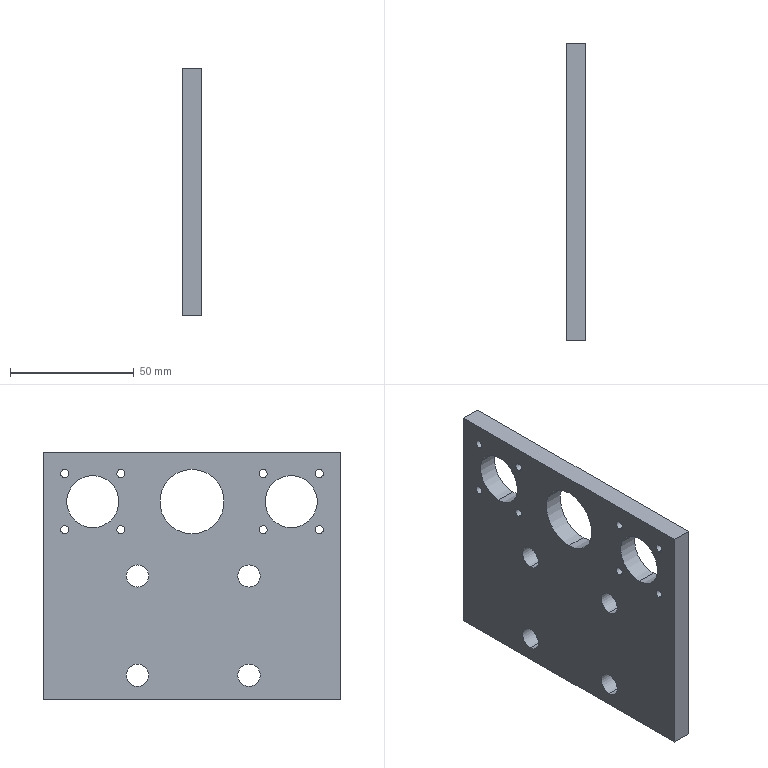Part | STEP file | X77B-01003 | 1 solid | 36 faces | box 8 x 120 x 100 mm | volume 83628 mm3 | cylinder 30 | plane 6 | commonest cylinder face diameters 3.3 x16 9 x8 21 x4 26 x2
STEP:
#1=CARTESIAN_POINT('',(289.016,-150.693,14.5));
#2=VERTEX_POINT('',#1);
#3=CARTESIAN_POINT('',(289.016,-150.693,5.5));
#4=VERTEX_POINT('',#3);
#5=CARTESIAN_POINT('',(289.016,-150.693,10.));
#6=DIRECTION('',(1.,0.,0.));
#7=DIRECTION('',(0.,0.,-1.));
#8=AXIS2_PLACEMENT_3D('',#5,#6,#7);
#9=CIRCLE('',#8,4.5);
#10=EDGE_CURVE('',#2,#4,#9,.T.);
#11=ORIENTED_EDGE('',*,*,#10,.F.);
#12=CARTESIAN_POINT('',(297.016,-150.693,14.5));
#13=VERTEX_POINT('',#12);
#14=CARTESIAN_POINT('',(297.016,-150.693,14.5));
#15=DIRECTION('',(1.,0.,0.));
#16=VECTOR('',#15,1000.);
#17=LINE('',#14,#16);
#18=EDGE_CURVE('',#2,#13,#17,.T.);
#19=ORIENTED_EDGE('',*,*,#18,.T.);
#20=CARTESIAN_POINT('',(297.016,-150.693,5.5));
#21=VERTEX_POINT('',#20);
#22=CARTESIAN_POINT('',(297.016,-150.693,10.));
#23=DIRECTION('',(1.,0.,0.));
#24=DIRECTION('',(0.,0.,-1.));
#25=AXIS2_PLACEMENT_3D('',#22,#23,#24);
#26=CIRCLE('',#25,4.5);
#27=EDGE_CURVE('',#13,#21,#26,.T.);
#28=ORIENTED_EDGE('',*,*,#27,.T.);
#29=CARTESIAN_POINT('',(297.016,-150.693,5.5));
#30=DIRECTION('',(1.,0.,0.));
#31=VECTOR('',#30,1000.);
#32=LINE('',#29,#31);
#33=EDGE_CURVE('',#4,#21,#32,.T.);
#34=ORIENTED_EDGE('',*,*,#33,.F.);
#35=EDGE_LOOP('',(#11,#19,#28,#34));
#36=FACE_OUTER_BOUND('',#35,.T.);
#37=CARTESIAN_POINT('',(297.016,-150.693,10.));
#38=DIRECTION('',(1.,0.,0.));
#39=DIRECTION('',(0.,0.,-1.));
#40=AXIS2_PLACEMENT_3D('',#37,#38,#39);
#41=CYLINDRICAL_SURFACE('',#40,4.5);
#42=ADVANCED_FACE('',(#36),#41,.F.);
#43=CARTESIAN_POINT('',(289.016,-150.693,54.5));
#44=VERTEX_POINT('',#43);
#45=CARTESIAN_POINT('',(289.016,-150.693,45.5));
#46=VERTEX_POINT('',#45);
#47=CARTESIAN_POINT('',(289.016,-150.693,50.));
#48=DIRECTION('',(1.,0.,0.));
#49=DIRECTION('',(0.,0.,-1.));
#50=AXIS2_PLACEMENT_3D('',#47,#48,#49);
#51=CIRCLE('',#50,4.5);
#52=EDGE_CURVE('',#44,#46,#51,.T.);
#53=ORIENTED_EDGE('',*,*,#52,.F.);
#54=CARTESIAN_POINT('',(297.016,-150.693,54.5));
#55=VERTEX_POINT('',#54);
#56=CARTESIAN_POINT('',(297.016,-150.693,54.5));
#57=DIRECTION('',(1.,0.,0.));
#58=VECTOR('',#57,1000.);
#59=LINE('',#56,#58);
#60=EDGE_CURVE('',#44,#55,#59,.T.);
#61=ORIENTED_EDGE('',*,*,#60,.T.);
#62=CARTESIAN_POINT('',(297.016,-150.693,45.5));
#63=VERTEX_POINT('',#62);
#64=CARTESIAN_POINT('',(297.016,-150.693,50.));
#65=DIRECTION('',(1.,0.,0.));
#66=DIRECTION('',(0.,0.,-1.));
#67=AXIS2_PLACEMENT_3D('',#64,#65,#66);
#68=CIRCLE('',#67,4.5);
#69=EDGE_CURVE('',#55,#63,#68,.T.);
#70=ORIENTED_EDGE('',*,*,#69,.T.);
#71=CARTESIAN_POINT('',(297.016,-150.693,45.5));
#72=DIRECTION('',(1.,0.,0.));
#73=VECTOR('',#72,1000.);
#74=LINE('',#71,#73);
#75=EDGE_CURVE('',#46,#63,#74,.T.);
#76=ORIENTED_EDGE('',*,*,#75,.F.);
#77=EDGE_LOOP('',(#53,#61,#70,#76));
#78=FACE_OUTER_BOUND('',#77,.T.);
#79=CARTESIAN_POINT('',(297.016,-150.693,50.));
#80=DIRECTION('',(1.,0.,0.));
#81=DIRECTION('',(0.,0.,-1.));
#82=AXIS2_PLACEMENT_3D('',#79,#80,#81);
#83=CYLINDRICAL_SURFACE('',#82,4.5);
#84=ADVANCED_FACE('',(#78),#83,.F.);
#85=CARTESIAN_POINT('',(289.016,-105.693,14.5));
#86=VERTEX_POINT('',#85);
#87=CARTESIAN_POINT('',(289.016,-105.693,5.5));
#88=VERTEX_POINT('',#87);
#89=CARTESIAN_POINT('',(289.016,-105.693,10.));
#90=DIRECTION('',(1.,0.,0.));
#91=DIRECTION('',(0.,0.,-1.));
#92=AXIS2_PLACEMENT_3D('',#89,#90,#91);
#93=CIRCLE('',#92,4.5);
#94=EDGE_CURVE('',#86,#88,#93,.T.);
#95=ORIENTED_EDGE('',*,*,#94,.F.);
#96=CARTESIAN_POINT('',(297.016,-105.693,14.5));
#97=VERTEX_POINT('',#96);
#98=CARTESIAN_POINT('',(297.016,-105.693,14.5));
#99=DIRECTION('',(1.,0.,0.));
#100=VECTOR('',#99,1000.);
#101=LINE('',#98,#100);
#102=EDGE_CURVE('',#86,#97,#101,.T.);
#103=ORIENTED_EDGE('',*,*,#102,.T.);
#104=CARTESIAN_POINT('',(297.016,-105.693,5.5));
#105=VERTEX_POINT('',#104);
#106=CARTESIAN_POINT('',(297.016,-105.693,10.));
#107=DIRECTION('',(1.,0.,0.));
#108=DIRECTION('',(0.,0.,-1.));
#109=AXIS2_PLACEMENT_3D('',#106,#107,#108);
#110=CIRCLE('',#109,4.5);
#111=EDGE_CURVE('',#97,#105,#110,.T.);
#112=ORIENTED_EDGE('',*,*,#111,.T.);
#113=CARTESIAN_POINT('',(297.016,-105.693,5.5));
#114=DIRECTION('',(1.,0.,0.));
#115=VECTOR('',#114,1000.);
#116=LINE('',#113,#115);
#117=EDGE_CURVE('',#88,#105,#116,.T.);
#118=ORIENTED_EDGE('',*,*,#117,.F.);
#119=EDGE_LOOP('',(#95,#103,#112,#118));
#120=FACE_OUTER_BOUND('',#119,.T.);
#121=CARTESIAN_POINT('',(297.016,-105.693,10.));
#122=DIRECTION('',(1.,0.,0.));
#123=DIRECTION('',(0.,0.,-1.));
#124=AXIS2_PLACEMENT_3D('',#121,#122,#123);
#125=CYLINDRICAL_SURFACE('',#124,4.5);
#126=ADVANCED_FACE('',(#120),#125,.F.);
#127=CARTESIAN_POINT('',(289.016,-105.693,54.5));
#128=VERTEX_POINT('',#127);
#129=CARTESIAN_POINT('',(289.016,-105.693,45.5));
#130=VERTEX_POINT('',#129);
#131=CARTESIAN_POINT('',(289.016,-105.693,50.));
#132=DIRECTION('',(1.,0.,0.));
#133=DIRECTION('',(0.,0.,-1.));
#134=AXIS2_PLACEMENT_3D('',#131,#132,#133);
#135=CIRCLE('',#134,4.5);
#136=EDGE_CURVE('',#128,#130,#135,.T.);
#137=ORIENTED_EDGE('',*,*,#136,.F.);
#138=CARTESIAN_POINT('',(297.016,-105.693,54.5));
#139=VERTEX_POINT('',#138);
#140=CARTESIAN_POINT('',(297.016,-105.693,54.5));
#141=DIRECTION('',(1.,0.,0.));
#142=VECTOR('',#141,1000.);
#143=LINE('',#140,#142);
#144=EDGE_CURVE('',#128,#139,#143,.T.);
#145=ORIENTED_EDGE('',*,*,#144,.T.);
#146=CARTESIAN_POINT('',(297.016,-105.693,45.5));
#147=VERTEX_POINT('',#146);
#148=CARTESIAN_POINT('',(297.016,-105.693,50.));
#149=DIRECTION('',(1.,0.,0.));
#150=DIRECTION('',(0.,0.,-1.));
#151=AXIS2_PLACEMENT_3D('',#148,#149,#150);
#152=CIRCLE('',#151,4.5);
#153=EDGE_CURVE('',#139,#147,#152,.T.);
#154=ORIENTED_EDGE('',*,*,#153,.T.);
#155=CARTESIAN_POINT('',(297.016,-105.693,45.5));
#156=DIRECTION('',(1.,0.,0.));
#157=VECTOR('',#156,1000.);
#158=LINE('',#155,#157);
#159=EDGE_CURVE('',#130,#147,#158,.T.);
#160=ORIENTED_EDGE('',*,*,#159,.F.);
#161=EDGE_LOOP('',(#137,#145,#154,#160));
#162=FACE_OUTER_BOUND('',#161,.T.);
#163=CARTESIAN_POINT('',(297.016,-105.693,50.));
#164=DIRECTION('',(1.,0.,0.));
#165=DIRECTION('',(0.,0.,-1.));
#166=AXIS2_PLACEMENT_3D('',#163,#164,#165);
#167=CYLINDRICAL_SURFACE('',#166,4.5);
#168=ADVANCED_FACE('',(#162),#167,.F.);
#169=CARTESIAN_POINT('',(289.016,-76.387,70.336));
#170=VERTEX_POINT('',#169);
#171=CARTESIAN_POINT('',(289.016,-76.387,67.036));
#172=VERTEX_POINT('',#171);
#173=CARTESIAN_POINT('',(289.016,-76.387,68.686));
#174=DIRECTION('',(1.,0.,0.));
#175=DIRECTION('',(0.,0.,-1.));
#176=AXIS2_PLACEMENT_3D('',#173,#174,#175);
#177=CIRCLE('',#176,1.65);
#178=EDGE_CURVE('',#170,#172,#177,.T.);
#179=ORIENTED_EDGE('',*,*,#178,.F.);
#180=CARTESIAN_POINT('',(297.016,-76.387,70.336));
#181=VERTEX_POINT('',#180);
#182=CARTESIAN_POINT('',(297.016,-76.387,70.336));
#183=DIRECTION('',(1.,0.,0.));
#184=VECTOR('',#183,1000.);
#185=LINE('',#182,#184);
#186=EDGE_CURVE('',#170,#181,#185,.T.);
#187=ORIENTED_EDGE('',*,*,#186,.T.);
#188=CARTESIAN_POINT('',(297.016,-76.387,67.036));
#189=VERTEX_POINT('',#188);
#190=CARTESIAN_POINT('',(297.016,-76.387,68.686));
#191=DIRECTION('',(1.,0.,0.));
#192=DIRECTION('',(0.,0.,-1.));
#193=AXIS2_PLACEMENT_3D('',#190,#191,#192);
#194=CIRCLE('',#193,1.65);
#195=EDGE_CURVE('',#181,#189,#194,.T.);
#196=ORIENTED_EDGE('',*,*,#195,.T.);
#197=CARTESIAN_POINT('',(297.016,-76.387,67.036));
#198=DIRECTION('',(1.,0.,0.));
#199=VECTOR('',#198,1000.);
#200=LINE('',#197,#199);
#201=EDGE_CURVE('',#172,#189,#200,.T.);
#202=ORIENTED_EDGE('',*,*,#201,.F.);
#203=EDGE_LOOP('',(#179,#187,#196,#202));
#204=FACE_OUTER_BOUND('',#203,.T.);
#205=CARTESIAN_POINT('',(297.016,-76.387,68.686));
#206=DIRECTION('',(1.,0.,0.));
#207=DIRECTION('',(0.,0.,-1.));
#208=AXIS2_PLACEMENT_3D('',#205,#206,#207);
#209=CYLINDRICAL_SURFACE('',#208,1.65);
#210=ADVANCED_FACE('',(#204),#209,.F.);
#211=CARTESIAN_POINT('',(289.016,-99.014,70.336));
#212=VERTEX_POINT('',#211);
#213=CARTESIAN_POINT('',(289.016,-99.014,67.036));
#214=VERTEX_POINT('',#213);
#215=CARTESIAN_POINT('',(289.016,-99.014,68.686));
#216=DIRECTION('',(1.,0.,0.));
#217=DIRECTION('',(0.,0.,-1.));
#218=AXIS2_PLACEMENT_3D('',#215,#216,#217);
#219=CIRCLE('',#218,1.65);
#220=EDGE_CURVE('',#212,#214,#219,.T.);
#221=ORIENTED_EDGE('',*,*,#220,.F.);
#222=CARTESIAN_POINT('',(297.016,-99.014,70.336));
#223=VERTEX_POINT('',#222);
#224=CARTESIAN_POINT('',(297.016,-99.014,70.336));
#225=DIRECTION('',(1.,0.,0.));
#226=VECTOR('',#225,1000.);
#227=LINE('',#224,#226);
#228=EDGE_CURVE('',#212,#223,#227,.T.);
#229=ORIENTED_EDGE('',*,*,#228,.T.);
#230=CARTESIAN_POINT('',(297.016,-99.014,67.036));
#231=VERTEX_POINT('',#230);
#232=CARTESIAN_POINT('',(297.016,-99.014,68.686));
#233=DIRECTION('',(1.,0.,0.));
#234=DIRECTION('',(0.,0.,-1.));
#235=AXIS2_PLACEMENT_3D('',#232,#233,#234);
#236=CIRCLE('',#235,1.65);
#237=EDGE_CURVE('',#223,#231,#236,.T.);
#238=ORIENTED_EDGE('',*,*,#237,.T.);
#239=CARTESIAN_POINT('',(297.016,-99.014,67.036));
#240=DIRECTION('',(1.,0.,0.));
#241=VECTOR('',#240,1000.);
#242=LINE('',#239,#241);
#243=EDGE_CURVE('',#214,#231,#242,.T.);
#244=ORIENTED_EDGE('',*,*,#243,.F.);
#245=EDGE_LOOP('',(#221,#229,#238,#244));
#246=FACE_OUTER_BOUND('',#245,.T.);
#247=CARTESIAN_POINT('',(297.016,-99.014,68.686));
#248=DIRECTION('',(1.,0.,0.));
#249=DIRECTION('',(0.,0.,-1.));
#250=AXIS2_PLACEMENT_3D('',#247,#248,#249);
#251=CYLINDRICAL_SURFACE('',#250,1.65);
#252=ADVANCED_FACE('',(#246),#251,.F.);
#253=CARTESIAN_POINT('',(289.016,-76.387,92.964));
#254=VERTEX_POINT('',#253);
#255=CARTESIAN_POINT('',(289.016,-76.387,89.664));
#256=VERTEX_POINT('',#255);
#257=CARTESIAN_POINT('',(289.016,-76.387,91.314));
#258=DIRECTION('',(1.,0.,0.));
#259=DIRECTION('',(0.,0.,-1.));
#260=AXIS2_PLACEMENT_3D('',#257,#258,#259);
#261=CIRCLE('',#260,1.65);
#262=EDGE_CURVE('',#254,#256,#261,.T.);
#263=ORIENTED_EDGE('',*,*,#262,.F.);
#264=CARTESIAN_POINT('',(297.016,-76.387,92.964));
#265=VERTEX_POINT('',#264);
#266=CARTESIAN_POINT('',(297.016,-76.387,92.964));
#267=DIRECTION('',(1.,0.,0.));
#268=VECTOR('',#267,1000.);
#269=LINE('',#266,#268);
#270=EDGE_CURVE('',#254,#265,#269,.T.);
#271=ORIENTED_EDGE('',*,*,#270,.T.);
#272=CARTESIAN_POINT('',(297.016,-76.387,89.664));
#273=VERTEX_POINT('',#272);
#274=CARTESIAN_POINT('',(297.016,-76.387,91.314));
#275=DIRECTION('',(1.,0.,0.));
#276=DIRECTION('',(0.,0.,-1.));
#277=AXIS2_PLACEMENT_3D('',#274,#275,#276);
#278=CIRCLE('',#277,1.65);
#279=EDGE_CURVE('',#265,#273,#278,.T.);
#280=ORIENTED_EDGE('',*,*,#279,.T.);
#281=CARTESIAN_POINT('',(297.016,-76.387,89.664));
#282=DIRECTION('',(1.,0.,0.));
#283=VECTOR('',#282,1000.);
#284=LINE('',#281,#283);
#285=EDGE_CURVE('',#256,#273,#284,.T.);
#286=ORIENTED_EDGE('',*,*,#285,.F.);
#287=EDGE_LOOP('',(#263,#271,#280,#286));
#288=FACE_OUTER_BOUND('',#287,.T.);
#289=CARTESIAN_POINT('',(297.016,-76.387,91.314));
#290=DIRECTION('',(1.,0.,0.));
#291=DIRECTION('',(0.,0.,-1.));
#292=AXIS2_PLACEMENT_3D('',#289,#290,#291);
#293=CYLINDRICAL_SURFACE('',#292,1.65);
#294=ADVANCED_FACE('',(#288),#293,.F.);
#295=CARTESIAN_POINT('',(289.016,-99.014,92.964));
#296=VERTEX_POINT('',#295);
#297=CARTESIAN_POINT('',(289.016,-99.014,89.664));
#298=VERTEX_POINT('',#297);
#299=CARTESIAN_POINT('',(289.016,-99.014,91.314));
#300=DIRECTION('',(1.,0.,0.));
#301=DIRECTION('',(0.,0.,-1.));
#302=AXIS2_PLACEMENT_3D('',#299,#300,#301);
#303=CIRCLE('',#302,1.65);
#304=EDGE_CURVE('',#296,#298,#303,.T.);
#305=ORIENTED_EDGE('',*,*,#304,.F.);
#306=CARTESIAN_POINT('',(297.016,-99.014,92.964));
#307=VERTEX_POINT('',#306);
#308=CARTESIAN_POINT('',(297.016,-99.014,92.964));
#309=DIRECTION('',(1.,0.,0.));
#310=VECTOR('',#309,1000.);
#311=LINE('',#308,#310);
#312=EDGE_CURVE('',#296,#307,#311,.T.);
#313=ORIENTED_EDGE('',*,*,#312,.T.);
#314=CARTESIAN_POINT('',(297.016,-99.014,89.664));
#315=VERTEX_POINT('',#314);
#316=CARTESIAN_POINT('',(297.016,-99.014,91.314));
#317=DIRECTION('',(1.,0.,0.));
#318=DIRECTION('',(0.,0.,-1.));
#319=AXIS2_PLACEMENT_3D('',#316,#317,#318);
#320=CIRCLE('',#319,1.65);
#321=EDGE_CURVE('',#307,#315,#320,.T.);
#322=ORIENTED_EDGE('',*,*,#321,.T.);
#323=CARTESIAN_POINT('',(297.016,-99.014,89.664));
#324=DIRECTION('',(1.,0.,0.));
#325=VECTOR('',#324,1000.);
#326=LINE('',#323,#325);
#327=EDGE_CURVE('',#298,#315,#326,.T.);
#328=ORIENTED_EDGE('',*,*,#327,.F.);
#329=EDGE_LOOP('',(#305,#313,#322,#328));
#330=FACE_OUTER_BOUND('',#329,.T.);
#331=CARTESIAN_POINT('',(297.016,-99.014,91.314));
#332=DIRECTION('',(1.,0.,0.));
#333=DIRECTION('',(0.,0.,-1.));
#334=AXIS2_PLACEMENT_3D('',#331,#332,#333);
#335=CYLINDRICAL_SURFACE('',#334,1.65);
#336=ADVANCED_FACE('',(#330),#335,.F.);
#337=CARTESIAN_POINT('',(289.016,-156.401,70.336));
#338=VERTEX_POINT('',#337);
#339=CARTESIAN_POINT('',(289.016,-156.401,67.036));
#340=VERTEX_POINT('',#339);
#341=CARTESIAN_POINT('',(289.016,-156.401,68.686));
#342=DIRECTION('',(1.,0.,0.));
#343=DIRECTION('',(0.,0.,-1.));
#344=AXIS2_PLACEMENT_3D('',#341,#342,#343);
#345=CIRCLE('',#344,1.65);
#346=EDGE_CURVE('',#338,#340,#345,.T.);
#347=ORIENTED_EDGE('',*,*,#346,.F.);
#348=CARTESIAN_POINT('',(297.016,-156.401,70.336));
#349=VERTEX_POINT('',#348);
#350=CARTESIAN_POINT('',(297.016,-156.401,70.336));
#351=DIRECTION('',(1.,0.,0.));
#352=VECTOR('',#351,1000.);
#353=LINE('',#350,#352);
#354=EDGE_CURVE('',#338,#349,#353,.T.);
#355=ORIENTED_EDGE('',*,*,#354,.T.);
#356=CARTESIAN_POINT('',(297.016,-156.401,67.036));
#357=VERTEX_POINT('',#356);
#358=CARTESIAN_POINT('',(297.016,-156.401,68.686));
#359=DIRECTION('',(1.,0.,0.));
#360=DIRECTION('',(0.,0.,-1.));
#361=AXIS2_PLACEMENT_3D('',#358,#359,#360);
#362=CIRCLE('',#361,1.65);
#363=EDGE_CURVE('',#349,#357,#362,.T.);
#364=ORIENTED_EDGE('',*,*,#363,.T.);
#365=CARTESIAN_POINT('',(297.016,-156.401,67.036));
#366=DIRECTION('',(1.,0.,0.));
#367=VECTOR('',#366,1000.);
#368=LINE('',#365,#367);
#369=EDGE_CURVE('',#340,#357,#368,.T.);
#370=ORIENTED_EDGE('',*,*,#369,.F.);
#371=EDGE_LOOP('',(#347,#355,#364,#370));
#372=FACE_OUTER_BOUND('',#371,.T.);
#373=CARTESIAN_POINT('',(297.016,-156.401,68.686));
#374=DIRECTION('',(1.,0.,0.));
#375=DIRECTION('',(0.,0.,-1.));
#376=AXIS2_PLACEMENT_3D('',#373,#374,#375);
#377=CYLINDRICAL_SURFACE('',#376,1.65);
#378=ADVANCED_FACE('',(#372),#377,.F.);
#379=CARTESIAN_POINT('',(289.016,-156.401,92.964));
#380=VERTEX_POINT('',#379);
#381=CARTESIAN_POINT('',(289.016,-156.401,89.664));
#382=VERTEX_POINT('',#381);
#383=CARTESIAN_POINT('',(289.016,-156.401,91.314));
#384=DIRECTION('',(1.,0.,0.));
#385=DIRECTION('',(0.,0.,-1.));
#386=AXIS2_PLACEMENT_3D('',#383,#384,#385);
#387=CIRCLE('',#386,1.65);
#388=EDGE_CURVE('',#380,#382,#387,.T.);
#389=ORIENTED_EDGE('',*,*,#388,.F.);
#390=CARTESIAN_POINT('',(297.016,-156.401,92.964));
#391=VERTEX_POINT('',#390);
#392=CARTESIAN_POINT('',(297.016,-156.401,92.964));
#393=DIRECTION('',(1.,0.,0.));
#394=VECTOR('',#393,1000.);
#395=LINE('',#392,#394);
#396=EDGE_CURVE('',#380,#391,#395,.T.);
#397=ORIENTED_EDGE('',*,*,#396,.T.);
#398=CARTESIAN_POINT('',(297.016,-156.401,89.664));
#399=VERTEX_POINT('',#398);
#400=CARTESIAN_POINT('',(297.016,-156.401,91.314));
#401=DIRECTION('',(1.,0.,0.));
#402=DIRECTION('',(0.,0.,-1.));
#403=AXIS2_PLACEMENT_3D('',#400,#401,#402);
#404=CIRCLE('',#403,1.65);
#405=EDGE_CURVE('',#391,#399,#404,.T.);
#406=ORIENTED_EDGE('',*,*,#405,.T.);
#407=CARTESIAN_POINT('',(297.016,-156.401,89.664));
#408=DIRECTION('',(1.,0.,0.));
#409=VECTOR('',#408,1000.);
#410=LINE('',#407,#409);
#411=EDGE_CURVE('',#382,#399,#410,.T.);
#412=ORIENTED_EDGE('',*,*,#411,.F.);
#413=EDGE_LOOP('',(#389,#397,#406,#412));
#414=FACE_OUTER_BOUND('',#413,.T.);
#415=CARTESIAN_POINT('',(297.016,-156.401,91.314));
#416=DIRECTION('',(1.,0.,0.));
#417=DIRECTION('',(0.,0.,-1.));
#418=AXIS2_PLACEMENT_3D('',#415,#416,#417);
#419=CYLINDRICAL_SURFACE('',#418,1.65);
#420=ADVANCED_FACE('',(#414),#419,.F.);
#421=CARTESIAN_POINT('',(289.016,-179.028,92.964));
#422=VERTEX_POINT('',#421);
#423=CARTESIAN_POINT('',(289.016,-179.028,89.664));
#424=VERTEX_POINT('',#423);
#425=CARTESIAN_POINT('',(289.016,-179.028,91.314));
#426=DIRECTION('',(1.,0.,0.));
#427=DIRECTION('',(0.,0.,-1.));
#428=AXIS2_PLACEMENT_3D('',#425,#426,#427);
#429=CIRCLE('',#428,1.65);
#430=EDGE_CURVE('',#422,#424,#429,.T.);
#431=ORIENTED_EDGE('',*,*,#430,.F.);
#432=CARTESIAN_POINT('',(297.016,-179.028,92.964));
#433=VERTEX_POINT('',#432);
#434=CARTESIAN_POINT('',(297.016,-179.028,92.964));
#435=DIRECTION('',(1.,0.,0.));
#436=VECTOR('',#435,1000.);
#437=LINE('',#434,#436);
#438=EDGE_CURVE('',#422,#433,#437,.T.);
#439=ORIENTED_EDGE('',*,*,#438,.T.);
#440=CARTESIAN_POINT('',(297.016,-179.028,89.664));
#441=VERTEX_POINT('',#440);
#442=CARTESIAN_POINT('',(297.016,-179.028,91.314));
#443=DIRECTION('',(1.,0.,0.));
#444=DIRECTION('',(0.,0.,-1.));
#445=AXIS2_PLACEMENT_3D('',#442,#443,#444);
#446=CIRCLE('',#445,1.65);
#447=EDGE_CURVE('',#433,#441,#446,.T.);
#448=ORIENTED_EDGE('',*,*,#447,.T.);
#449=CARTESIAN_POINT('',(297.016,-179.028,89.664));
#450=DIRECTION('',(1.,0.,0.));
#451=VECTOR('',#450,1000.);
#452=LINE('',#449,#451);
#453=EDGE_CURVE('',#424,#441,#452,.T.);
#454=ORIENTED_EDGE('',*,*,#453,.F.);
#455=EDGE_LOOP('',(#431,#439,#448,#454));
#456=FACE_OUTER_BOUND('',#455,.T.);
#457=CARTESIAN_POINT('',(297.016,-179.028,91.314));
#458=DIRECTION('',(1.,0.,0.));
#459=DIRECTION('',(0.,0.,-1.));
#460=AXIS2_PLACEMENT_3D('',#457,#458,#459);
#461=CYLINDRICAL_SURFACE('',#460,1.65);
#462=ADVANCED_FACE('',(#456),#461,.F.);
#463=CARTESIAN_POINT('',(289.016,-179.028,70.336));
#464=VERTEX_POINT('',#463);
#465=CARTESIAN_POINT('',(289.016,-179.028,67.036));
#466=VERTEX_POINT('',#465);
#467=CARTESIAN_POINT('',(289.016,-179.028,68.686));
#468=DIRECTION('',(1.,0.,0.));
#469=DIRECTION('',(0.,0.,-1.));
#470=AXIS2_PLACEMENT_3D('',#467,#468,#469);
#471=CIRCLE('',#470,1.65);
#472=EDGE_CURVE('',#464,#466,#471,.T.);
#473=ORIENTED_EDGE('',*,*,#472,.F.);
#474=CARTESIAN_POINT('',(297.016,-179.028,70.336));
#475=VERTEX_POINT('',#474);
#476=CARTESIAN_POINT('',(297.016,-179.028,70.336));
#477=DIRECTION('',(1.,0.,0.));
#478=VECTOR('',#477,1000.);
#479=LINE('',#476,#478);
#480=EDGE_CURVE('',#464,#475,#479,.T.);
#481=ORIENTED_EDGE('',*,*,#480,.T.);
#482=CARTESIAN_POINT('',(297.016,-179.028,67.036));
#483=VERTEX_POINT('',#482);
#484=CARTESIAN_POINT('',(297.016,-179.028,68.686));
#485=DIRECTION('',(1.,0.,0.));
#486=DIRECTION('',(0.,0.,-1.));
#487=AXIS2_PLACEMENT_3D('',#484,#485,#486);
#488=CIRCLE('',#487,1.65);
#489=EDGE_CURVE('',#475,#483,#488,.T.);
#490=ORIENTED_EDGE('',*,*,#489,.T.);
#491=CARTESIAN_POINT('',(297.016,-179.028,67.036));
#492=DIRECTION('',(1.,0.,0.));
#493=VECTOR('',#492,1000.);
#494=LINE('',#491,#493);
#495=EDGE_CURVE('',#466,#483,#494,.T.);
#496=ORIENTED_EDGE('',*,*,#495,.F.);
#497=EDGE_LOOP('',(#473,#481,#490,#496));
#498=FACE_OUTER_BOUND('',#497,.T.);
#499=CARTESIAN_POINT('',(297.016,-179.028,68.686));
#500=DIRECTION('',(1.,0.,0.));
#501=DIRECTION('',(0.,0.,-1.));
#502=AXIS2_PLACEMENT_3D('',#499,#500,#501);
#503=CYLINDRICAL_SURFACE('',#502,1.65);
#504=ADVANCED_FACE('',(#498),#503,.F.);
#505=CARTESIAN_POINT('',(289.016,-167.7,90.5));
#506=VERTEX_POINT('',#505);
#507=CARTESIAN_POINT('',(289.016,-167.7,69.5));
#508=VERTEX_POINT('',#507);
#509=CARTESIAN_POINT('',(289.016,-167.7,80.));
#510=DIRECTION('',(1.,0.,0.));
#511=DIRECTION('',(0.,0.,-1.));
#512=AXIS2_PLACEMENT_3D('',#509,#510,#511);
#513=CIRCLE('',#512,10.5);
#514=EDGE_CURVE('',#506,#508,#513,.T.);
#515=ORIENTED_EDGE('',*,*,#514,.F.);
#516=CARTESIAN_POINT('',(297.016,-167.7,90.5));
#517=VERTEX_POINT('',#516);
#518=CARTESIAN_POINT('',(289.016,-167.7,90.5));
#519=DIRECTION('',(1.,0.,0.));
#520=VECTOR('',#519,1000.);
#521=LINE('',#518,#520);
#522=EDGE_CURVE('',#506,#517,#521,.T.);
#523=ORIENTED_EDGE('',*,*,#522,.T.);
#524=CARTESIAN_POINT('',(297.016,-167.7,69.5));
#525=VERTEX_POINT('',#524);
#526=CARTESIAN_POINT('',(297.016,-167.7,80.));
#527=DIRECTION('',(1.,0.,0.));
#528=DIRECTION('',(0.,0.,-1.));
#529=AXIS2_PLACEMENT_3D('',#526,#527,#528);
#530=CIRCLE('',#529,10.5);
#531=EDGE_CURVE('',#517,#525,#530,.T.);
#532=ORIENTED_EDGE('',*,*,#531,.T.);
#533=CARTESIAN_POINT('',(289.016,-167.7,69.5));
#534=DIRECTION('',(1.,0.,0.));
#535=VECTOR('',#534,1000.);
#536=LINE('',#533,#535);
#537=EDGE_CURVE('',#508,#525,#536,.T.);
#538=ORIENTED_EDGE('',*,*,#537,.F.);
#539=EDGE_LOOP('',(#515,#523,#532,#538));
#540=FACE_OUTER_BOUND('',#539,.T.);
#541=CARTESIAN_POINT('',(289.016,-167.7,80.));
#542=DIRECTION('',(1.,0.,0.));
#543=DIRECTION('',(0.,0.,-1.));
#544=AXIS2_PLACEMENT_3D('',#541,#542,#543);
#545=CYLINDRICAL_SURFACE('',#544,10.5);
#546=ADVANCED_FACE('',(#540),#545,.F.);
#547=CARTESIAN_POINT('',(289.016,-87.7,90.5));
#548=VERTEX_POINT('',#547);
#549=CARTESIAN_POINT('',(289.016,-87.7,69.5));
#550=VERTEX_POINT('',#549);
#551=CARTESIAN_POINT('',(289.016,-87.7,80.));
#552=DIRECTION('',(1.,0.,0.));
#553=DIRECTION('',(0.,0.,-1.));
#554=AXIS2_PLACEMENT_3D('',#551,#552,#553);
#555=CIRCLE('',#554,10.5);
#556=EDGE_CURVE('',#548,#550,#555,.T.);
#557=ORIENTED_EDGE('',*,*,#556,.F.);
#558=CARTESIAN_POINT('',(297.016,-87.7,90.5));
#559=VERTEX_POINT('',#558);
#560=CARTESIAN_POINT('',(289.016,-87.7,90.5));
#561=DIRECTION('',(1.,0.,0.));
#562=VECTOR('',#561,1000.);
#563=LINE('',#560,#562);
#564=EDGE_CURVE('',#548,#559,#563,.T.);
#565=ORIENTED_EDGE('',*,*,#564,.T.);
#566=CARTESIAN_POINT('',(297.016,-87.7,69.5));
#567=VERTEX_POINT('',#566);
#568=CARTESIAN_POINT('',(297.016,-87.7,80.));
#569=DIRECTION('',(1.,0.,0.));
#570=DIRECTION('',(0.,0.,-1.));
#571=AXIS2_PLACEMENT_3D('',#568,#569,#570);
#572=CIRCLE('',#571,10.5);
#573=EDGE_CURVE('',#559,#567,#572,.T.);
#574=ORIENTED_EDGE('',*,*,#573,.T.);
#575=CARTESIAN_POINT('',(289.016,-87.7,69.5));
#576=DIRECTION('',(1.,0.,0.));
#577=VECTOR('',#576,1000.);
#578=LINE('',#575,#577);
#579=EDGE_CURVE('',#550,#567,#578,.T.);
#580=ORIENTED_EDGE('',*,*,#579,.F.);
#581=EDGE_LOOP('',(#557,#565,#574,#580));
#582=FACE_OUTER_BOUND('',#581,.T.);
#583=CARTESIAN_POINT('',(289.016,-87.7,80.));
#584=DIRECTION('',(1.,0.,0.));
#585=DIRECTION('',(0.,0.,-1.));
#586=AXIS2_PLACEMENT_3D('',#583,#584,#585);
#587=CYLINDRICAL_SURFACE('',#586,10.5);
#588=ADVANCED_FACE('',(#582),#587,.F.);
#589=CARTESIAN_POINT('',(289.016,-127.7,93.));
#590=VERTEX_POINT('',#589);
#591=CARTESIAN_POINT('',(289.016,-127.7,67.));
#592=VERTEX_POINT('',#591);
#593=CARTESIAN_POINT('',(289.016,-127.7,80.));
#594=DIRECTION('',(1.,0.,0.));
#595=DIRECTION('',(0.,0.,-1.));
#596=AXIS2_PLACEMENT_3D('',#593,#594,#595);
#597=CIRCLE('',#596,13.);
#598=EDGE_CURVE('',#590,#592,#597,.T.);
#599=ORIENTED_EDGE('',*,*,#598,.F.);
#600=CARTESIAN_POINT('',(297.016,-127.7,93.));
#601=VERTEX_POINT('',#600);
#602=CARTESIAN_POINT('',(289.016,-127.7,93.));
#603=DIRECTION('',(1.,0.,0.));
#604=VECTOR('',#603,1000.);
#605=LINE('',#602,#604);
#606=EDGE_CURVE('',#590,#601,#605,.T.);
#607=ORIENTED_EDGE('',*,*,#606,.T.);
#608=CARTESIAN_POINT('',(297.016,-127.7,67.));
#609=VERTEX_POINT('',#608);
#610=CARTESIAN_POINT('',(297.016,-127.7,80.));
#611=DIRECTION('',(1.,0.,0.));
#612=DIRECTION('',(0.,0.,-1.));
#613=AXIS2_PLACEMENT_3D('',#610,#611,#612);
#614=CIRCLE('',#613,13.);
#615=EDGE_CURVE('',#601,#609,#614,.T.);
#616=ORIENTED_EDGE('',*,*,#615,.T.);
#617=CARTESIAN_POINT('',(289.016,-127.7,67.));
#618=DIRECTION('',(1.,0.,0.));
#619=VECTOR('',#618,1000.);
#620=LINE('',#617,#619);
#621=EDGE_CURVE('',#592,#609,#620,.T.);
#622=ORIENTED_EDGE('',*,*,#621,.F.);
#623=EDGE_LOOP('',(#599,#607,#616,#622));
#624=FACE_OUTER_BOUND('',#623,.T.);
#625=CARTESIAN_POINT('',(289.016,-127.7,80.));
#626=DIRECTION('',(1.,0.,0.));
#627=DIRECTION('',(0.,0.,-1.));
#628=AXIS2_PLACEMENT_3D('',#625,#626,#627);
#629=CYLINDRICAL_SURFACE('',#628,13.);
#630=ADVANCED_FACE('',(#624),#629,.F.);
#631=CARTESIAN_POINT('',(297.016,-150.693,10.));
#632=DIRECTION('',(1.,0.,0.));
#633=DIRECTION('',(0.,0.,-1.));
#634=AXIS2_PLACEMENT_3D('',#631,#632,#633);
#635=CIRCLE('',#634,4.5);
#636=EDGE_CURVE('',#21,#13,#635,.T.);
#637=ORIENTED_EDGE('',*,*,#636,.F.);
#638=ORIENTED_EDGE('',*,*,#27,.F.);
#639=EDGE_LOOP('',(#637,#638));
#640=FACE_BOUND('',#639,.T.);
#641=CARTESIAN_POINT('',(297.016,-150.693,50.));
#642=DIRECTION('',(1.,0.,0.));
#643=DIRECTION('',(0.,0.,-1.));
#644=AXIS2_PLACEMENT_3D('',#641,#642,#643);
#645=CIRCLE('',#644,4.5);
#646=EDGE_CURVE('',#63,#55,#645,.T.);
#647=ORIENTED_EDGE('',*,*,#646,.F.);
#648=ORIENTED_EDGE('',*,*,#69,.F.);
#649=EDGE_LOOP('',(#647,#648));
#650=FACE_BOUND('',#649,.T.);
#651=CARTESIAN_POINT('',(297.016,-105.693,10.));
#652=DIRECTION('',(1.,0.,0.));
#653=DIRECTION('',(0.,0.,-1.));
#654=AXIS2_PLACEMENT_3D('',#651,#652,#653);
#655=CIRCLE('',#654,4.5);
#656=EDGE_CURVE('',#105,#97,#655,.T.);
#657=ORIENTED_EDGE('',*,*,#656,.F.);
#658=ORIENTED_EDGE('',*,*,#111,.F.);
#659=EDGE_LOOP('',(#657,#658));
#660=FACE_BOUND('',#659,.T.);
#661=CARTESIAN_POINT('',(297.016,-105.693,50.));
#662=DIRECTION('',(1.,0.,0.));
#663=DIRECTION('',(0.,0.,-1.));
#664=AXIS2_PLACEMENT_3D('',#661,#662,#663);
#665=CIRCLE('',#664,4.5);
#666=EDGE_CURVE('',#147,#139,#665,.T.);
#667=ORIENTED_EDGE('',*,*,#666,.F.);
#668=ORIENTED_EDGE('',*,*,#153,.F.);
#669=EDGE_LOOP('',(#667,#668));
#670=FACE_BOUND('',#669,.T.);
#671=CARTESIAN_POINT('',(297.016,-76.387,68.686));
#672=DIRECTION('',(1.,0.,0.));
#673=DIRECTION('',(0.,0.,-1.));
#674=AXIS2_PLACEMENT_3D('',#671,#672,#673);
#675=CIRCLE('',#674,1.65);
#676=EDGE_CURVE('',#189,#181,#675,.T.);
#677=ORIENTED_EDGE('',*,*,#676,.F.);
#678=ORIENTED_EDGE('',*,*,#195,.F.);
#679=EDGE_LOOP('',(#677,#678));
#680=FACE_BOUND('',#679,.T.);
#681=CARTESIAN_POINT('',(297.016,-99.014,68.686));
#682=DIRECTION('',(1.,0.,0.));
#683=DIRECTION('',(0.,0.,-1.));
#684=AXIS2_PLACEMENT_3D('',#681,#682,#683);
#685=CIRCLE('',#684,1.65);
#686=EDGE_CURVE('',#231,#223,#685,.T.);
#687=ORIENTED_EDGE('',*,*,#686,.F.);
#688=ORIENTED_EDGE('',*,*,#237,.F.);
#689=EDGE_LOOP('',(#687,#688));
#690=FACE_BOUND('',#689,.T.);
#691=CARTESIAN_POINT('',(297.016,-76.387,91.314));
#692=DIRECTION('',(1.,0.,0.));
#693=DIRECTION('',(0.,0.,-1.));
#694=AXIS2_PLACEMENT_3D('',#691,#692,#693);
#695=CIRCLE('',#694,1.65);
#696=EDGE_CURVE('',#273,#265,#695,.T.);
#697=ORIENTED_EDGE('',*,*,#696,.F.);
#698=ORIENTED_EDGE('',*,*,#279,.F.);
#699=EDGE_LOOP('',(#697,#698));
#700=FACE_BOUND('',#699,.T.);
#701=CARTESIAN_POINT('',(297.016,-99.014,91.314));
#702=DIRECTION('',(1.,0.,0.));
#703=DIRECTION('',(0.,0.,-1.));
#704=AXIS2_PLACEMENT_3D('',#701,#702,#703);
#705=CIRCLE('',#704,1.65);
#706=EDGE_CURVE('',#315,#307,#705,.T.);
#707=ORIENTED_EDGE('',*,*,#706,.F.);
#708=ORIENTED_EDGE('',*,*,#321,.F.);
#709=EDGE_LOOP('',(#707,#708));
#710=FACE_BOUND('',#709,.T.);
#711=CARTESIAN_POINT('',(297.016,-156.401,68.686));
#712=DIRECTION('',(1.,0.,0.));
#713=DIRECTION('',(0.,0.,-1.));
#714=AXIS2_PLACEMENT_3D('',#711,#712,#713);
#715=CIRCLE('',#714,1.65);
#716=EDGE_CURVE('',#357,#349,#715,.T.);
#717=ORIENTED_EDGE('',*,*,#716,.F.);
#718=ORIENTED_EDGE('',*,*,#363,.F.);
#719=EDGE_LOOP('',(#717,#718));
#720=FACE_BOUND('',#719,.T.);
#721=CARTESIAN_POINT('',(297.016,-156.401,91.314));
#722=DIRECTION('',(1.,0.,0.));
#723=DIRECTION('',(0.,0.,-1.));
#724=AXIS2_PLACEMENT_3D('',#721,#722,#723);
#725=CIRCLE('',#724,1.65);
#726=EDGE_CURVE('',#399,#391,#725,.T.);
#727=ORIENTED_EDGE('',*,*,#726,.F.);
#728=ORIENTED_EDGE('',*,*,#405,.F.);
#729=EDGE_LOOP('',(#727,#728));
#730=FACE_BOUND('',#729,.T.);
#731=CARTESIAN_POINT('',(297.016,-179.028,91.314));
#732=DIRECTION('',(1.,0.,0.));
#733=DIRECTION('',(0.,0.,-1.));
#734=AXIS2_PLACEMENT_3D('',#731,#732,#733);
#735=CIRCLE('',#734,1.65);
#736=EDGE_CURVE('',#441,#433,#735,.T.);
#737=ORIENTED_EDGE('',*,*,#736,.F.);
#738=ORIENTED_EDGE('',*,*,#447,.F.);
#739=EDGE_LOOP('',(#737,#738));
#740=FACE_BOUND('',#739,.T.);
#741=CARTESIAN_POINT('',(297.016,-179.028,68.686));
#742=DIRECTION('',(1.,0.,0.));
#743=DIRECTION('',(0.,0.,-1.));
#744=AXIS2_PLACEMENT_3D('',#741,#742,#743);
#745=CIRCLE('',#744,1.65);
#746=EDGE_CURVE('',#483,#475,#745,.T.);
#747=ORIENTED_EDGE('',*,*,#746,.F.);
#748=ORIENTED_EDGE('',*,*,#489,.F.);
#749=EDGE_LOOP('',(#747,#748));
#750=FACE_BOUND('',#749,.T.);
#751=CARTESIAN_POINT('',(297.016,-167.7,80.));
#752=DIRECTION('',(1.,0.,0.));
#753=DIRECTION('',(0.,0.,-1.));
#754=AXIS2_PLACEMENT_3D('',#751,#752,#753);
#755=CIRCLE('',#754,10.5);
#756=EDGE_CURVE('',#525,#517,#755,.T.);
#757=ORIENTED_EDGE('',*,*,#756,.F.);
#758=ORIENTED_EDGE('',*,*,#531,.F.);
#759=EDGE_LOOP('',(#757,#758));
#760=FACE_BOUND('',#759,.T.);
#761=CARTESIAN_POINT('',(297.016,-87.7,80.));
#762=DIRECTION('',(1.,0.,0.));
#763=DIRECTION('',(0.,0.,-1.));
#764=AXIS2_PLACEMENT_3D('',#761,#762,#763);
#765=CIRCLE('',#764,10.5);
#766=EDGE_CURVE('',#567,#559,#765,.T.);
#767=ORIENTED_EDGE('',*,*,#766,.F.);
#768=ORIENTED_EDGE('',*,*,#573,.F.);
#769=EDGE_LOOP('',(#767,#768));
#770=FACE_BOUND('',#769,.T.);
#771=CARTESIAN_POINT('',(297.016,-127.7,80.));
#772=DIRECTION('',(1.,0.,0.));
#773=DIRECTION('',(0.,0.,-1.));
#774=AXIS2_PLACEMENT_3D('',#771,#772,#773);
#775=CIRCLE('',#774,13.);
#776=EDGE_CURVE('',#609,#601,#775,.T.);
#777=ORIENTED_EDGE('',*,*,#776,.F.);
#778=ORIENTED_EDGE('',*,*,#615,.F.);
#779=EDGE_LOOP('',(#777,#778));
#780=FACE_BOUND('',#779,.T.);
#781=CARTESIAN_POINT('',(297.016,-187.7,0.));
#782=VERTEX_POINT('',#781);
#783=CARTESIAN_POINT('',(297.016,-67.7,0.));
#784=VERTEX_POINT('',#783);
#785=CARTESIAN_POINT('',(297.016,-67.7,0.));
#786=DIRECTION('',(0.,1.,0.));
#787=VECTOR('',#786,1000.);
#788=LINE('',#785,#787);
#789=EDGE_CURVE('',#782,#784,#788,.T.);
#790=ORIENTED_EDGE('',*,*,#789,.T.);
#791=CARTESIAN_POINT('',(297.016,-67.7,100.));
#792=VERTEX_POINT('',#791);
#793=CARTESIAN_POINT('',(297.016,-67.7,100.));
#794=DIRECTION('',(0.,0.,-1.));
#795=VECTOR('',#794,1000.);
#796=LINE('',#793,#795);
#797=EDGE_CURVE('',#792,#784,#796,.T.);
#798=ORIENTED_EDGE('',*,*,#797,.F.);
#799=CARTESIAN_POINT('',(297.016,-187.7,100.));
#800=VERTEX_POINT('',#799);
#801=CARTESIAN_POINT('',(297.016,-67.7,100.));
#802=DIRECTION('',(0.,1.,0.));
#803=VECTOR('',#802,1000.);
#804=LINE('',#801,#803);
#805=EDGE_CURVE('',#800,#792,#804,.T.);
#806=ORIENTED_EDGE('',*,*,#805,.F.);
#807=CARTESIAN_POINT('',(297.016,-187.7,100.));
#808=DIRECTION('',(0.,0.,-1.));
#809=VECTOR('',#808,1000.);
#810=LINE('',#807,#809);
#811=EDGE_CURVE('',#800,#782,#810,.T.);
#812=ORIENTED_EDGE('',*,*,#811,.T.);
#813=EDGE_LOOP('',(#790,#798,#806,#812));
#814=FACE_OUTER_BOUND('',#813,.T.);
#815=CARTESIAN_POINT('',(297.016,-67.7,100.));
#816=DIRECTION('',(-1.,0.,0.));
#817=DIRECTION('',(0.,0.,1.));
#818=AXIS2_PLACEMENT_3D('',#815,#816,#817);
#819=PLANE('',#818);
#820=ADVANCED_FACE('',(#640,#650,#660,#670,#680,#690,#700,#710,#720,#730,#740,#750,#760,#770,#780,#814),#819,.F.);
#821=CARTESIAN_POINT('',(289.016,-67.7,0.));
#822=VERTEX_POINT('',#821);
#823=CARTESIAN_POINT('',(297.016,-67.7,0.));
#824=DIRECTION('',(-1.,0.,0.));
#825=VECTOR('',#824,1000.);
#826=LINE('',#823,#825);
#827=EDGE_CURVE('',#784,#822,#826,.T.);
#828=ORIENTED_EDGE('',*,*,#827,.T.);
#829=CARTESIAN_POINT('',(289.016,-67.7,100.));
#830=VERTEX_POINT('',#829);
#831=CARTESIAN_POINT('',(289.016,-67.7,100.));
#832=DIRECTION('',(0.,0.,-1.));
#833=VECTOR('',#832,1000.);
#834=LINE('',#831,#833);
#835=EDGE_CURVE('',#830,#822,#834,.T.);
#836=ORIENTED_EDGE('',*,*,#835,.F.);
#837=CARTESIAN_POINT('',(297.016,-67.7,100.));
#838=DIRECTION('',(-1.,0.,0.));
#839=VECTOR('',#838,1000.);
#840=LINE('',#837,#839);
#841=EDGE_CURVE('',#792,#830,#840,.T.);
#842=ORIENTED_EDGE('',*,*,#841,.F.);
#843=ORIENTED_EDGE('',*,*,#797,.T.);
#844=EDGE_LOOP('',(#828,#836,#842,#843));
#845=FACE_OUTER_BOUND('',#844,.T.);
#846=CARTESIAN_POINT('',(297.016,-67.7,100.));
#847=DIRECTION('',(0.,-1.,0.));
#848=DIRECTION('',(0.,0.,-1.));
#849=AXIS2_PLACEMENT_3D('',#846,#847,#848);
#850=PLANE('',#849);
#851=ADVANCED_FACE('',(#845),#850,.F.);
#852=CARTESIAN_POINT('',(289.016,-150.693,10.));
#853=DIRECTION('',(1.,0.,0.));
#854=DIRECTION('',(0.,0.,-1.));
#855=AXIS2_PLACEMENT_3D('',#852,#853,#854);
#856=CIRCLE('',#855,4.5);
#857=EDGE_CURVE('',#4,#2,#856,.T.);
#858=ORIENTED_EDGE('',*,*,#857,.T.);
#859=ORIENTED_EDGE('',*,*,#10,.T.);
#860=EDGE_LOOP('',(#858,#859));
#861=FACE_BOUND('',#860,.T.);
#862=CARTESIAN_POINT('',(289.016,-150.693,50.));
#863=DIRECTION('',(1.,0.,0.));
#864=DIRECTION('',(0.,0.,-1.));
#865=AXIS2_PLACEMENT_3D('',#862,#863,#864);
#866=CIRCLE('',#865,4.5);
#867=EDGE_CURVE('',#46,#44,#866,.T.);
#868=ORIENTED_EDGE('',*,*,#867,.T.);
#869=ORIENTED_EDGE('',*,*,#52,.T.);
#870=EDGE_LOOP('',(#868,#869));
#871=FACE_BOUND('',#870,.T.);
#872=CARTESIAN_POINT('',(289.016,-105.693,10.));
#873=DIRECTION('',(1.,0.,0.));
#874=DIRECTION('',(0.,0.,-1.));
#875=AXIS2_PLACEMENT_3D('',#872,#873,#874);
#876=CIRCLE('',#875,4.5);
#877=EDGE_CURVE('',#88,#86,#876,.T.);
#878=ORIENTED_EDGE('',*,*,#877,.T.);
#879=ORIENTED_EDGE('',*,*,#94,.T.);
#880=EDGE_LOOP('',(#878,#879));
#881=FACE_BOUND('',#880,.T.);
#882=CARTESIAN_POINT('',(289.016,-105.693,50.));
#883=DIRECTION('',(1.,0.,0.));
#884=DIRECTION('',(0.,0.,-1.));
#885=AXIS2_PLACEMENT_3D('',#882,#883,#884);
#886=CIRCLE('',#885,4.5);
#887=EDGE_CURVE('',#130,#128,#886,.T.);
#888=ORIENTED_EDGE('',*,*,#887,.T.);
#889=ORIENTED_EDGE('',*,*,#136,.T.);
#890=EDGE_LOOP('',(#888,#889));
#891=FACE_BOUND('',#890,.T.);
#892=CARTESIAN_POINT('',(289.016,-76.387,68.686));
#893=DIRECTION('',(1.,0.,0.));
#894=DIRECTION('',(0.,0.,-1.));
#895=AXIS2_PLACEMENT_3D('',#892,#893,#894);
#896=CIRCLE('',#895,1.65);
#897=EDGE_CURVE('',#172,#170,#896,.T.);
#898=ORIENTED_EDGE('',*,*,#897,.T.);
#899=ORIENTED_EDGE('',*,*,#178,.T.);
#900=EDGE_LOOP('',(#898,#899));
#901=FACE_BOUND('',#900,.T.);
#902=CARTESIAN_POINT('',(289.016,-99.014,68.686));
#903=DIRECTION('',(1.,0.,0.));
#904=DIRECTION('',(0.,0.,-1.));
#905=AXIS2_PLACEMENT_3D('',#902,#903,#904);
#906=CIRCLE('',#905,1.65);
#907=EDGE_CURVE('',#214,#212,#906,.T.);
#908=ORIENTED_EDGE('',*,*,#907,.T.);
#909=ORIENTED_EDGE('',*,*,#220,.T.);
#910=EDGE_LOOP('',(#908,#909));
#911=FACE_BOUND('',#910,.T.);
#912=CARTESIAN_POINT('',(289.016,-76.387,91.314));
#913=DIRECTION('',(1.,0.,0.));
#914=DIRECTION('',(0.,0.,-1.));
#915=AXIS2_PLACEMENT_3D('',#912,#913,#914);
#916=CIRCLE('',#915,1.65);
#917=EDGE_CURVE('',#256,#254,#916,.T.);
#918=ORIENTED_EDGE('',*,*,#917,.T.);
#919=ORIENTED_EDGE('',*,*,#262,.T.);
#920=EDGE_LOOP('',(#918,#919));
#921=FACE_BOUND('',#920,.T.);
#922=CARTESIAN_POINT('',(289.016,-99.014,91.314));
#923=DIRECTION('',(1.,0.,0.));
#924=DIRECTION('',(0.,0.,-1.));
#925=AXIS2_PLACEMENT_3D('',#922,#923,#924);
#926=CIRCLE('',#925,1.65);
#927=EDGE_CURVE('',#298,#296,#926,.T.);
#928=ORIENTED_EDGE('',*,*,#927,.T.);
#929=ORIENTED_EDGE('',*,*,#304,.T.);
#930=EDGE_LOOP('',(#928,#929));
#931=FACE_BOUND('',#930,.T.);
#932=CARTESIAN_POINT('',(289.016,-156.401,68.686));
#933=DIRECTION('',(1.,0.,0.));
#934=DIRECTION('',(0.,0.,-1.));
#935=AXIS2_PLACEMENT_3D('',#932,#933,#934);
#936=CIRCLE('',#935,1.65);
#937=EDGE_CURVE('',#340,#338,#936,.T.);
#938=ORIENTED_EDGE('',*,*,#937,.T.);
#939=ORIENTED_EDGE('',*,*,#346,.T.);
#940=EDGE_LOOP('',(#938,#939));
#941=FACE_BOUND('',#940,.T.);
#942=CARTESIAN_POINT('',(289.016,-156.401,91.314));
#943=DIRECTION('',(1.,0.,0.));
#944=DIRECTION('',(0.,0.,-1.));
#945=AXIS2_PLACEMENT_3D('',#942,#943,#944);
#946=CIRCLE('',#945,1.65);
#947=EDGE_CURVE('',#382,#380,#946,.T.);
#948=ORIENTED_EDGE('',*,*,#947,.T.);
#949=ORIENTED_EDGE('',*,*,#388,.T.);
#950=EDGE_LOOP('',(#948,#949));
#951=FACE_BOUND('',#950,.T.);
#952=CARTESIAN_POINT('',(289.016,-179.028,91.314));
#953=DIRECTION('',(1.,0.,0.));
#954=DIRECTION('',(0.,0.,-1.));
#955=AXIS2_PLACEMENT_3D('',#952,#953,#954);
#956=CIRCLE('',#955,1.65);
#957=EDGE_CURVE('',#424,#422,#956,.T.);
#958=ORIENTED_EDGE('',*,*,#957,.T.);
#959=ORIENTED_EDGE('',*,*,#430,.T.);
#960=EDGE_LOOP('',(#958,#959));
#961=FACE_BOUND('',#960,.T.);
#962=CARTESIAN_POINT('',(289.016,-179.028,68.686));
#963=DIRECTION('',(1.,0.,0.));
#964=DIRECTION('',(0.,0.,-1.));
#965=AXIS2_PLACEMENT_3D('',#962,#963,#964);
#966=CIRCLE('',#965,1.65);
#967=EDGE_CURVE('',#466,#464,#966,.T.);
#968=ORIENTED_EDGE('',*,*,#967,.T.);
#969=ORIENTED_EDGE('',*,*,#472,.T.);
#970=EDGE_LOOP('',(#968,#969));
#971=FACE_BOUND('',#970,.T.);
#972=CARTESIAN_POINT('',(289.016,-167.7,80.));
#973=DIRECTION('',(1.,0.,0.));
#974=DIRECTION('',(0.,0.,-1.));
#975=AXIS2_PLACEMENT_3D('',#972,#973,#974);
#976=CIRCLE('',#975,10.5);
#977=EDGE_CURVE('',#508,#506,#976,.T.);
#978=ORIENTED_EDGE('',*,*,#977,.T.);
#979=ORIENTED_EDGE('',*,*,#514,.T.);
#980=EDGE_LOOP('',(#978,#979));
#981=FACE_BOUND('',#980,.T.);
#982=CARTESIAN_POINT('',(289.016,-87.7,80.));
#983=DIRECTION('',(1.,0.,0.));
#984=DIRECTION('',(0.,0.,-1.));
#985=AXIS2_PLACEMENT_3D('',#982,#983,#984);
#986=CIRCLE('',#985,10.5);
#987=EDGE_CURVE('',#550,#548,#986,.T.);
#988=ORIENTED_EDGE('',*,*,#987,.T.);
#989=ORIENTED_EDGE('',*,*,#556,.T.);
#990=EDGE_LOOP('',(#988,#989));
#991=FACE_BOUND('',#990,.T.);
#992=CARTESIAN_POINT('',(289.016,-127.7,80.));
#993=DIRECTION('',(1.,0.,0.));
#994=DIRECTION('',(0.,0.,-1.));
#995=AXIS2_PLACEMENT_3D('',#992,#993,#994);
#996=CIRCLE('',#995,13.);
#997=EDGE_CURVE('',#592,#590,#996,.T.);
#998=ORIENTED_EDGE('',*,*,#997,.T.);
#999=ORIENTED_EDGE('',*,*,#598,.T.);
#1000=EDGE_LOOP('',(#998,#999));
#1001=FACE_BOUND('',#1000,.T.);
#1002=CARTESIAN_POINT('',(289.016,-187.7,0.));
#1003=VERTEX_POINT('',#1002);
#1004=CARTESIAN_POINT('',(289.016,-67.7,0.));
#1005=DIRECTION('',(0.,-1.,0.));
#1006=VECTOR('',#1005,1000.);
#1007=LINE('',#1004,#1006);
#1008=EDGE_CURVE('',#822,#1003,#1007,.T.);
#1009=ORIENTED_EDGE('',*,*,#1008,.T.);
#1010=CARTESIAN_POINT('',(289.016,-187.7,100.));
#1011=VERTEX_POINT('',#1010);
#1012=CARTESIAN_POINT('',(289.016,-187.7,100.));
#1013=DIRECTION('',(0.,0.,-1.));
#1014=VECTOR('',#1013,1000.);
#1015=LINE('',#1012,#1014);
#1016=EDGE_CURVE('',#1011,#1003,#1015,.T.);
#1017=ORIENTED_EDGE('',*,*,#1016,.F.);
#1018=CARTESIAN_POINT('',(289.016,-67.7,100.));
#1019=DIRECTION('',(0.,-1.,0.));
#1020=VECTOR('',#1019,1000.);
#1021=LINE('',#1018,#1020);
#1022=EDGE_CURVE('',#830,#1011,#1021,.T.);
#1023=ORIENTED_EDGE('',*,*,#1022,.F.);
#1024=ORIENTED_EDGE('',*,*,#835,.T.);
#1025=EDGE_LOOP('',(#1009,#1017,#1023,#1024));
#1026=FACE_OUTER_BOUND('',#1025,.T.);
#1027=CARTESIAN_POINT('',(289.016,-67.7,100.));
#1028=DIRECTION('',(1.,0.,0.));
#1029=DIRECTION('',(0.,0.,-1.));
#1030=AXIS2_PLACEMENT_3D('',#1027,#1028,#1029);
#1031=PLANE('',#1030);
#1032=ADVANCED_FACE('',(#861,#871,#881,#891,#901,#911,#921,#931,#941,#951,#961,#971,#981,#991,#1001,#1026),#1031,.F.);
#1033=CARTESIAN_POINT('',(297.016,-187.7,0.));
#1034=DIRECTION('',(1.,0.,0.));
#1035=VECTOR('',#1034,1000.);
#1036=LINE('',#1033,#1035);
#1037=EDGE_CURVE('',#1003,#782,#1036,.T.);
#1038=ORIENTED_EDGE('',*,*,#1037,.T.);
#1039=ORIENTED_EDGE('',*,*,#811,.F.);
#1040=CARTESIAN_POINT('',(297.016,-187.7,100.));
#1041=DIRECTION('',(1.,0.,0.));
#1042=VECTOR('',#1041,1000.);
#1043=LINE('',#1040,#1042);
#1044=EDGE_CURVE('',#1011,#800,#1043,.T.);
#1045=ORIENTED_EDGE('',*,*,#1044,.F.);
#1046=ORIENTED_EDGE('',*,*,#1016,.T.);
#1047=EDGE_LOOP('',(#1038,#1039,#1045,#1046));
#1048=FACE_OUTER_BOUND('',#1047,.T.);
#1049=CARTESIAN_POINT('',(297.016,-187.7,100.));
#1050=DIRECTION('',(0.,1.,0.));
#1051=DIRECTION('',(0.,0.,1.));
#1052=AXIS2_PLACEMENT_3D('',#1049,#1050,#1051);
#1053=PLANE('',#1052);
#1054=ADVANCED_FACE('',(#1048),#1053,.F.);
#1055=ORIENTED_EDGE('',*,*,#805,.T.);
#1056=ORIENTED_EDGE('',*,*,#841,.T.);
#1057=ORIENTED_EDGE('',*,*,#1022,.T.);
#1058=ORIENTED_EDGE('',*,*,#1044,.T.);
#1059=EDGE_LOOP('',(#1055,#1056,#1057,#1058));
#1060=FACE_OUTER_BOUND('',#1059,.T.);
#1061=CARTESIAN_POINT('',(297.016,-187.7,100.));
#1062=DIRECTION('',(0.,0.,-1.));
#1063=DIRECTION('',(-1.,0.,0.));
#1064=AXIS2_PLACEMENT_3D('',#1061,#1062,#1063);
#1065=PLANE('',#1064);
#1066=ADVANCED_FACE('',(#1060),#1065,.F.);
#1067=ORIENTED_EDGE('',*,*,#789,.F.);
#1068=ORIENTED_EDGE('',*,*,#1037,.F.);
#1069=ORIENTED_EDGE('',*,*,#1008,.F.);
#1070=ORIENTED_EDGE('',*,*,#827,.F.);
#1071=EDGE_LOOP('',(#1067,#1068,#1069,#1070));
#1072=FACE_OUTER_BOUND('',#1071,.T.);
#1073=CARTESIAN_POINT('',(297.016,-187.7,0.));
#1074=DIRECTION('',(0.,0.,-1.));
#1075=DIRECTION('',(-1.,0.,0.));
#1076=AXIS2_PLACEMENT_3D('',#1073,#1074,#1075);
#1077=PLANE('',#1076);
#1078=ADVANCED_FACE('',(#1072),#1077,.T.);
#1079=ORIENTED_EDGE('',*,*,#606,.F.);
#1080=ORIENTED_EDGE('',*,*,#997,.F.);
#1081=ORIENTED_EDGE('',*,*,#621,.T.);
#1082=ORIENTED_EDGE('',*,*,#776,.T.);
#1083=EDGE_LOOP('',(#1079,#1080,#1081,#1082));
#1084=FACE_OUTER_BOUND('',#1083,.T.);
#1085=CARTESIAN_POINT('',(289.016,-127.7,80.));
#1086=DIRECTION('',(1.,0.,0.));
#1087=DIRECTION('',(0.,0.,-1.));
#1088=AXIS2_PLACEMENT_3D('',#1085,#1086,#1087);
#1089=CYLINDRICAL_SURFACE('',#1088,13.);
#1090=ADVANCED_FACE('',(#1084),#1089,.F.);
#1091=ORIENTED_EDGE('',*,*,#564,.F.);
#1092=ORIENTED_EDGE('',*,*,#987,.F.);
#1093=ORIENTED_EDGE('',*,*,#579,.T.);
#1094=ORIENTED_EDGE('',*,*,#766,.T.);
#1095=EDGE_LOOP('',(#1091,#1092,#1093,#1094));
#1096=FACE_OUTER_BOUND('',#1095,.T.);
#1097=CARTESIAN_POINT('',(289.016,-87.7,80.));
#1098=DIRECTION('',(1.,0.,0.));
#1099=DIRECTION('',(0.,0.,-1.));
#1100=AXIS2_PLACEMENT_3D('',#1097,#1098,#1099);
#1101=CYLINDRICAL_SURFACE('',#1100,10.5);
#1102=ADVANCED_FACE('',(#1096),#1101,.F.);
#1103=ORIENTED_EDGE('',*,*,#522,.F.);
#1104=ORIENTED_EDGE('',*,*,#977,.F.);
#1105=ORIENTED_EDGE('',*,*,#537,.T.);
#1106=ORIENTED_EDGE('',*,*,#756,.T.);
#1107=EDGE_LOOP('',(#1103,#1104,#1105,#1106));
#1108=FACE_OUTER_BOUND('',#1107,.T.);
#1109=CARTESIAN_POINT('',(289.016,-167.7,80.));
#1110=DIRECTION('',(1.,0.,0.));
#1111=DIRECTION('',(0.,0.,-1.));
#1112=AXIS2_PLACEMENT_3D('',#1109,#1110,#1111);
#1113=CYLINDRICAL_SURFACE('',#1112,10.5);
#1114=ADVANCED_FACE('',(#1108),#1113,.F.);
#1115=ORIENTED_EDGE('',*,*,#480,.F.);
#1116=ORIENTED_EDGE('',*,*,#967,.F.);
#1117=ORIENTED_EDGE('',*,*,#495,.T.);
#1118=ORIENTED_EDGE('',*,*,#746,.T.);
#1119=EDGE_LOOP('',(#1115,#1116,#1117,#1118));
#1120=FACE_OUTER_BOUND('',#1119,.T.);
#1121=CARTESIAN_POINT('',(297.016,-179.028,68.686));
#1122=DIRECTION('',(1.,0.,0.));
#1123=DIRECTION('',(0.,0.,-1.));
#1124=AXIS2_PLACEMENT_3D('',#1121,#1122,#1123);
#1125=CYLINDRICAL_SURFACE('',#1124,1.65);
#1126=ADVANCED_FACE('',(#1120),#1125,.F.);
#1127=ORIENTED_EDGE('',*,*,#438,.F.);
#1128=ORIENTED_EDGE('',*,*,#957,.F.);
#1129=ORIENTED_EDGE('',*,*,#453,.T.);
#1130=ORIENTED_EDGE('',*,*,#736,.T.);
#1131=EDGE_LOOP('',(#1127,#1128,#1129,#1130));
#1132=FACE_OUTER_BOUND('',#1131,.T.);
#1133=CARTESIAN_POINT('',(297.016,-179.028,91.314));
#1134=DIRECTION('',(1.,0.,0.));
#1135=DIRECTION('',(0.,0.,-1.));
#1136=AXIS2_PLACEMENT_3D('',#1133,#1134,#1135);
#1137=CYLINDRICAL_SURFACE('',#1136,1.65);
#1138=ADVANCED_FACE('',(#1132),#1137,.F.);
#1139=ORIENTED_EDGE('',*,*,#396,.F.);
#1140=ORIENTED_EDGE('',*,*,#947,.F.);
#1141=ORIENTED_EDGE('',*,*,#411,.T.);
#1142=ORIENTED_EDGE('',*,*,#726,.T.);
#1143=EDGE_LOOP('',(#1139,#1140,#1141,#1142));
#1144=FACE_OUTER_BOUND('',#1143,.T.);
#1145=CARTESIAN_POINT('',(297.016,-156.401,91.314));
#1146=DIRECTION('',(1.,0.,0.));
#1147=DIRECTION('',(0.,0.,-1.));
#1148=AXIS2_PLACEMENT_3D('',#1145,#1146,#1147);
#1149=CYLINDRICAL_SURFACE('',#1148,1.65);
#1150=ADVANCED_FACE('',(#1144),#1149,.F.);
#1151=ORIENTED_EDGE('',*,*,#354,.F.);
#1152=ORIENTED_EDGE('',*,*,#937,.F.);
#1153=ORIENTED_EDGE('',*,*,#369,.T.);
#1154=ORIENTED_EDGE('',*,*,#716,.T.);
#1155=EDGE_LOOP('',(#1151,#1152,#1153,#1154));
#1156=FACE_OUTER_BOUND('',#1155,.T.);
#1157=CARTESIAN_POINT('',(297.016,-156.401,68.686));
#1158=DIRECTION('',(1.,0.,0.));
#1159=DIRECTION('',(0.,0.,-1.));
#1160=AXIS2_PLACEMENT_3D('',#1157,#1158,#1159);
#1161=CYLINDRICAL_SURFACE('',#1160,1.65);
#1162=ADVANCED_FACE('',(#1156),#1161,.F.);
#1163=ORIENTED_EDGE('',*,*,#312,.F.);
#1164=ORIENTED_EDGE('',*,*,#927,.F.);
#1165=ORIENTED_EDGE('',*,*,#327,.T.);
#1166=ORIENTED_EDGE('',*,*,#706,.T.);
#1167=EDGE_LOOP('',(#1163,#1164,#1165,#1166));
#1168=FACE_OUTER_BOUND('',#1167,.T.);
#1169=CARTESIAN_POINT('',(297.016,-99.014,91.314));
#1170=DIRECTION('',(1.,0.,0.));
#1171=DIRECTION('',(0.,0.,-1.));
#1172=AXIS2_PLACEMENT_3D('',#1169,#1170,#1171);
#1173=CYLINDRICAL_SURFACE('',#1172,1.65);
#1174=ADVANCED_FACE('',(#1168),#1173,.F.);
#1175=ORIENTED_EDGE('',*,*,#270,.F.);
#1176=ORIENTED_EDGE('',*,*,#917,.F.);
#1177=ORIENTED_EDGE('',*,*,#285,.T.);
#1178=ORIENTED_EDGE('',*,*,#696,.T.);
#1179=EDGE_LOOP('',(#1175,#1176,#1177,#1178));
#1180=FACE_OUTER_BOUND('',#1179,.T.);
#1181=CARTESIAN_POINT('',(297.016,-76.387,91.314));
#1182=DIRECTION('',(1.,0.,0.));
#1183=DIRECTION('',(0.,0.,-1.));
#1184=AXIS2_PLACEMENT_3D('',#1181,#1182,#1183);
#1185=CYLINDRICAL_SURFACE('',#1184,1.65);
#1186=ADVANCED_FACE('',(#1180),#1185,.F.);
#1187=ORIENTED_EDGE('',*,*,#228,.F.);
#1188=ORIENTED_EDGE('',*,*,#907,.F.);
#1189=ORIENTED_EDGE('',*,*,#243,.T.);
#1190=ORIENTED_EDGE('',*,*,#686,.T.);
#1191=EDGE_LOOP('',(#1187,#1188,#1189,#1190));
#1192=FACE_OUTER_BOUND('',#1191,.T.);
#1193=CARTESIAN_POINT('',(297.016,-99.014,68.686));
#1194=DIRECTION('',(1.,0.,0.));
#1195=DIRECTION('',(0.,0.,-1.));
#1196=AXIS2_PLACEMENT_3D('',#1193,#1194,#1195);
#1197=CYLINDRICAL_SURFACE('',#1196,1.65);
#1198=ADVANCED_FACE('',(#1192),#1197,.F.);
#1199=ORIENTED_EDGE('',*,*,#186,.F.);
#1200=ORIENTED_EDGE('',*,*,#897,.F.);
#1201=ORIENTED_EDGE('',*,*,#201,.T.);
#1202=ORIENTED_EDGE('',*,*,#676,.T.);
#1203=EDGE_LOOP('',(#1199,#1200,#1201,#1202));
#1204=FACE_OUTER_BOUND('',#1203,.T.);
#1205=CARTESIAN_POINT('',(297.016,-76.387,68.686));
#1206=DIRECTION('',(1.,0.,0.));
#1207=DIRECTION('',(0.,0.,-1.));
#1208=AXIS2_PLACEMENT_3D('',#1205,#1206,#1207);
#1209=CYLINDRICAL_SURFACE('',#1208,1.65);
#1210=ADVANCED_FACE('',(#1204),#1209,.F.);
#1211=ORIENTED_EDGE('',*,*,#144,.F.);
#1212=ORIENTED_EDGE('',*,*,#887,.F.);
#1213=ORIENTED_EDGE('',*,*,#159,.T.);
#1214=ORIENTED_EDGE('',*,*,#666,.T.);
#1215=EDGE_LOOP('',(#1211,#1212,#1213,#1214));
#1216=FACE_OUTER_BOUND('',#1215,.T.);
#1217=CARTESIAN_POINT('',(297.016,-105.693,50.));
#1218=DIRECTION('',(1.,0.,0.));
#1219=DIRECTION('',(0.,0.,-1.));
#1220=AXIS2_PLACEMENT_3D('',#1217,#1218,#1219);
#1221=CYLINDRICAL_SURFACE('',#1220,4.5);
#1222=ADVANCED_FACE('',(#1216),#1221,.F.);
#1223=ORIENTED_EDGE('',*,*,#102,.F.);
#1224=ORIENTED_EDGE('',*,*,#877,.F.);
#1225=ORIENTED_EDGE('',*,*,#117,.T.);
#1226=ORIENTED_EDGE('',*,*,#656,.T.);
#1227=EDGE_LOOP('',(#1223,#1224,#1225,#1226));
#1228=FACE_OUTER_BOUND('',#1227,.T.);
#1229=CARTESIAN_POINT('',(297.016,-105.693,10.));
#1230=DIRECTION('',(1.,0.,0.));
#1231=DIRECTION('',(0.,0.,-1.));
#1232=AXIS2_PLACEMENT_3D('',#1229,#1230,#1231);
#1233=CYLINDRICAL_SURFACE('',#1232,4.5);
#1234=ADVANCED_FACE('',(#1228),#1233,.F.);
#1235=ORIENTED_EDGE('',*,*,#60,.F.);
#1236=ORIENTED_EDGE('',*,*,#867,.F.);
#1237=ORIENTED_EDGE('',*,*,#75,.T.);
#1238=ORIENTED_EDGE('',*,*,#646,.T.);
#1239=EDGE_LOOP('',(#1235,#1236,#1237,#1238));
#1240=FACE_OUTER_BOUND('',#1239,.T.);
#1241=CARTESIAN_POINT('',(297.016,-150.693,50.));
#1242=DIRECTION('',(1.,0.,0.));
#1243=DIRECTION('',(0.,0.,-1.));
#1244=AXIS2_PLACEMENT_3D('',#1241,#1242,#1243);
#1245=CYLINDRICAL_SURFACE('',#1244,4.5);
#1246=ADVANCED_FACE('',(#1240),#1245,.F.);
#1247=ORIENTED_EDGE('',*,*,#18,.F.);
#1248=ORIENTED_EDGE('',*,*,#857,.F.);
#1249=ORIENTED_EDGE('',*,*,#33,.T.);
#1250=ORIENTED_EDGE('',*,*,#636,.T.);
#1251=EDGE_LOOP('',(#1247,#1248,#1249,#1250));
#1252=FACE_OUTER_BOUND('',#1251,.T.);
#1253=CARTESIAN_POINT('',(297.016,-150.693,10.));
#1254=DIRECTION('',(1.,0.,0.));
#1255=DIRECTION('',(0.,0.,-1.));
#1256=AXIS2_PLACEMENT_3D('',#1253,#1254,#1255);
#1257=CYLINDRICAL_SURFACE('',#1256,4.5);
#1258=ADVANCED_FACE('',(#1252),#1257,.F.);
#1259=CLOSED_SHELL('',(#42,#84,#126,#168,#210,#252,#294,#336,#378,#420,#462,#504,#546,#588,#630,#820,#851,#1032,#1054,#1066,#1078,#1090,#1102,#1114,#1126,#1138,#1150,#1162,#1174,#1186,#1198,#1210,#1222,#1234,#1246,#1258));
#1260=MANIFOLD_SOLID_BREP('',#1259);
#1261=CARTESIAN_POINT('',(0.,0.,0.));
#1262=DIRECTION('',(0.,0.,1.));
#1263=DIRECTION('',(1.,0.,0.));
#1264=AXIS2_PLACEMENT_3D('',#1261,#1262,#1263);
#1265=(LENGTH_UNIT()NAMED_UNIT(*)SI_UNIT(.MILLI.,.METRE.));
#1266=UNCERTAINTY_MEASURE_WITH_UNIT(LENGTH_MEASURE(0.00001),#1265,'','');
#1267=(NAMED_UNIT(*)PLANE_ANGLE_UNIT()SI_UNIT($,.RADIAN.));
#1268=(NAMED_UNIT(*)SI_UNIT($,.STERADIAN.)SOLID_ANGLE_UNIT());
#1269=(GEOMETRIC_REPRESENTATION_CONTEXT(3)GLOBAL_UNCERTAINTY_ASSIGNED_CONTEXT((#1266))GLOBAL_UNIT_ASSIGNED_CONTEXT((#1265,#1267,#1268))REPRESENTATION_CONTEXT('',''));
#1270=ADVANCED_BREP_SHAPE_REPRESENTATION('',(#1260,#1264),#1269);